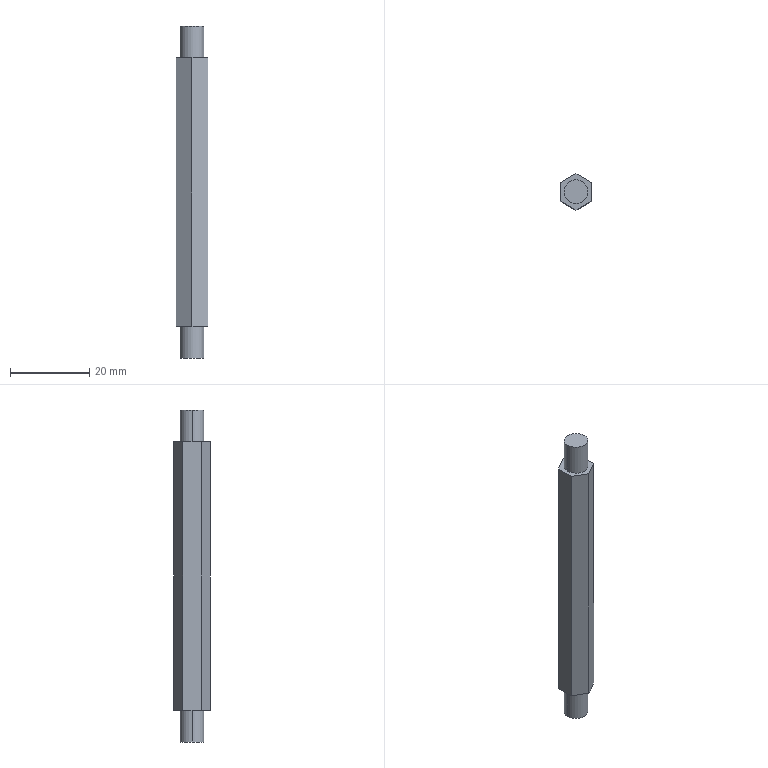Part | STEP file | 1 solid | 14 faces | box 8 x 9.238 x 84 mm | volume 4221 mm3 | plane 10 | cylinder 4 | commonest cylinder face diameters 6 x4
STEP:
#1=CARTESIAN_POINT('',(0.,0.,0.));
#2=DIRECTION('',(0.,0.,1.));
#3=DIRECTION('',(1.,0.,0.));
#4=AXIS2_PLACEMENT_3D('',#1,#2,#3);
#5=CARTESIAN_POINT('',(-5.42,-20.574,-52.535));
#6=VERTEX_POINT('',#5);
#7=CARTESIAN_POINT('',(-11.42,-20.574,-52.535));
#8=VERTEX_POINT('',#7);
#9=CARTESIAN_POINT('',(-8.42,-20.574,-52.535));
#10=DIRECTION('',(0.,0.,1.));
#11=DIRECTION('',(-1.,0.,0.));
#12=AXIS2_PLACEMENT_3D('',#9,#10,#11);
#13=CIRCLE('',#12,3.);
#14=CARTESIAN_POINT('',(-8.42,-20.574,-52.535));
#15=DIRECTION('',(0.,0.,-1.));
#16=DIRECTION('',(-1.,0.,0.));
#17=AXIS2_PLACEMENT_3D('',#14,#15,#16);
#18=CYLINDRICAL_SURFACE('',#17,3.);
#19=CARTESIAN_POINT('',(6.283,0.));
#20=DIRECTION('',(-1.,0.));
#21=VECTOR('',#20,1.);
#22=LINE('',#19,#21);
#23=(GEOMETRIC_REPRESENTATION_CONTEXT(2)PARAMETRIC_REPRESENTATION_CONTEXT()REPRESENTATION_CONTEXT('',''));
#24=DEFINITIONAL_REPRESENTATION('',(#22),#23);
#25=PCURVE('',#18,#24);
#26=CARTESIAN_POINT('',(-8.42,-20.574,-52.535));
#27=DIRECTION('',(0.,0.,-1.));
#28=DIRECTION('',(-1.,0.,0.));
#29=AXIS2_PLACEMENT_3D('',#26,#27,#28);
#30=PLANE('',#29);
#31=CARTESIAN_POINT('',(3.,0.));
#32=CARTESIAN_POINT('',(3.,-5.196));
#33=CARTESIAN_POINT('',(-1.5,-2.598));
#34=CARTESIAN_POINT('',(-6.,0.));
#35=CARTESIAN_POINT('',(-1.5,2.598));
#36=CARTESIAN_POINT('',(3.,5.196));
#37=CARTESIAN_POINT('',(3.,0.));
#38=(BOUNDED_CURVE()B_SPLINE_CURVE(2,(#31,#32,#33,#34,#35,#36,#37),.UNSPECIFIED.,.T.,.F.)B_SPLINE_CURVE_WITH_KNOTS((1,2,2,2,2,1),(-2.094,0.,2.094,4.189,6.283,8.378),.UNSPECIFIED.)CURVE()GEOMETRIC_REPRESENTATION_ITEM()RATIONAL_B_SPLINE_CURVE((1.,0.5,1.,0.5,1.,0.5,1.))REPRESENTATION_ITEM(''));
#39=(GEOMETRIC_REPRESENTATION_CONTEXT(2)PARAMETRIC_REPRESENTATION_CONTEXT()REPRESENTATION_CONTEXT('',''));
#40=DEFINITIONAL_REPRESENTATION('',(#38),#39);
#41=PCURVE('',#30,#40);
#42=SURFACE_CURVE('',#13,(#25,#41),.PCURVE_S1.);
#43=EDGE_CURVE('',#6,#8,#42,.T.);
#44=ORIENTED_EDGE('',*,*,#43,.F.);
#45=CARTESIAN_POINT('',(-5.42,-20.574,-60.535));
#46=VERTEX_POINT('',#45);
#47=CARTESIAN_POINT('',(-5.42,-20.574,-52.535));
#48=DIRECTION('',(0.,0.,-1.));
#49=VECTOR('',#48,1.);
#50=LINE('',#47,#49);
#51=CARTESIAN_POINT('',(3.142,0.));
#52=DIRECTION('',(0.,1.));
#53=VECTOR('',#52,1.);
#54=LINE('',#51,#53);
#55=(GEOMETRIC_REPRESENTATION_CONTEXT(2)PARAMETRIC_REPRESENTATION_CONTEXT()REPRESENTATION_CONTEXT('',''));
#56=DEFINITIONAL_REPRESENTATION('',(#54),#55);
#57=PCURVE('',#18,#56);
#58=CARTESIAN_POINT('',(-8.42,-20.574,-52.535));
#59=DIRECTION('',(0.,0.,-1.));
#60=DIRECTION('',(-1.,0.,0.));
#61=AXIS2_PLACEMENT_3D('',#58,#59,#60);
#62=CYLINDRICAL_SURFACE('',#61,3.);
#63=CARTESIAN_POINT('',(3.142,0.));
#64=DIRECTION('',(0.,1.));
#65=VECTOR('',#64,1.);
#66=LINE('',#63,#65);
#67=(GEOMETRIC_REPRESENTATION_CONTEXT(2)PARAMETRIC_REPRESENTATION_CONTEXT()REPRESENTATION_CONTEXT('',''));
#68=DEFINITIONAL_REPRESENTATION('',(#66),#67);
#69=PCURVE('',#62,#68);
#70=SURFACE_CURVE('',#50,(#57,#69),.PCURVE_S1.);
#71=EDGE_CURVE('',#6,#46,#70,.T.);
#72=ORIENTED_EDGE('',*,*,#71,.T.);
#73=CARTESIAN_POINT('',(-11.42,-20.574,-60.535));
#74=VERTEX_POINT('',#73);
#75=CARTESIAN_POINT('',(-8.42,-20.574,-60.535));
#76=DIRECTION('',(0.,0.,1.));
#77=DIRECTION('',(-1.,0.,0.));
#78=AXIS2_PLACEMENT_3D('',#75,#76,#77);
#79=CIRCLE('',#78,3.);
#80=CARTESIAN_POINT('',(6.283,8.));
#81=DIRECTION('',(-1.,0.));
#82=VECTOR('',#81,1.);
#83=LINE('',#80,#82);
#84=(GEOMETRIC_REPRESENTATION_CONTEXT(2)PARAMETRIC_REPRESENTATION_CONTEXT()REPRESENTATION_CONTEXT('',''));
#85=DEFINITIONAL_REPRESENTATION('',(#83),#84);
#86=PCURVE('',#18,#85);
#87=CARTESIAN_POINT('',(-8.42,-20.574,-60.535));
#88=DIRECTION('',(0.,0.,-1.));
#89=DIRECTION('',(0.,1.,0.));
#90=AXIS2_PLACEMENT_3D('',#87,#88,#89);
#91=PLANE('',#90);
#92=CARTESIAN_POINT('',(0.,-3.));
#93=CARTESIAN_POINT('',(-5.196,-3.));
#94=CARTESIAN_POINT('',(-2.598,1.5));
#95=CARTESIAN_POINT('',(0.,6.));
#96=CARTESIAN_POINT('',(2.598,1.5));
#97=CARTESIAN_POINT('',(5.196,-3.));
#98=CARTESIAN_POINT('',(0.,-3.));
#99=(BOUNDED_CURVE()B_SPLINE_CURVE(2,(#92,#93,#94,#95,#96,#97,#98),.UNSPECIFIED.,.T.,.F.)B_SPLINE_CURVE_WITH_KNOTS((1,2,2,2,2,1),(-2.094,0.,2.094,4.189,6.283,8.378),.UNSPECIFIED.)CURVE()GEOMETRIC_REPRESENTATION_ITEM()RATIONAL_B_SPLINE_CURVE((1.,0.5,1.,0.5,1.,0.5,1.))REPRESENTATION_ITEM(''));
#100=(GEOMETRIC_REPRESENTATION_CONTEXT(2)PARAMETRIC_REPRESENTATION_CONTEXT()REPRESENTATION_CONTEXT('',''));
#101=DEFINITIONAL_REPRESENTATION('',(#99),#100);
#102=PCURVE('',#91,#101);
#103=SURFACE_CURVE('',#79,(#86,#102),.PCURVE_S1.);
#104=EDGE_CURVE('',#46,#74,#103,.T.);
#105=ORIENTED_EDGE('',*,*,#104,.T.);
#106=CARTESIAN_POINT('',(-11.42,-20.574,-52.535));
#107=DIRECTION('',(0.,0.,-1.));
#108=VECTOR('',#107,1.);
#109=LINE('',#106,#108);
#110=CARTESIAN_POINT('',(0.,0.));
#111=DIRECTION('',(0.,1.));
#112=VECTOR('',#111,1.);
#113=LINE('',#110,#112);
#114=(GEOMETRIC_REPRESENTATION_CONTEXT(2)PARAMETRIC_REPRESENTATION_CONTEXT()REPRESENTATION_CONTEXT('',''));
#115=DEFINITIONAL_REPRESENTATION('',(#113),#114);
#116=PCURVE('',#18,#115);
#117=CARTESIAN_POINT('',(6.283,0.));
#118=DIRECTION('',(0.,1.));
#119=VECTOR('',#118,1.);
#120=LINE('',#117,#119);
#121=(GEOMETRIC_REPRESENTATION_CONTEXT(2)PARAMETRIC_REPRESENTATION_CONTEXT()REPRESENTATION_CONTEXT('',''));
#122=DEFINITIONAL_REPRESENTATION('',(#120),#121);
#123=PCURVE('',#62,#122);
#124=SURFACE_CURVE('',#109,(#116,#123),.PCURVE_S1.);
#125=EDGE_CURVE('',#8,#74,#124,.T.);
#126=ORIENTED_EDGE('',*,*,#125,.F.);
#127=EDGE_LOOP('',(#44,#72,#105,#126));
#128=FACE_BOUND('',#127,.T.);
#129=ADVANCED_FACE('',(#128),#18,.T.);
#130=CARTESIAN_POINT('',(-11.42,-20.574,23.465));
#131=VERTEX_POINT('',#130);
#132=CARTESIAN_POINT('',(-5.42,-20.574,23.465));
#133=VERTEX_POINT('',#132);
#134=CARTESIAN_POINT('',(-8.42,-20.574,23.465));
#135=DIRECTION('',(0.,0.,-1.));
#136=DIRECTION('',(-1.,0.,0.));
#137=AXIS2_PLACEMENT_3D('',#134,#135,#136);
#138=CIRCLE('',#137,3.);
#139=CARTESIAN_POINT('',(-8.42,-20.574,15.465));
#140=DIRECTION('',(0.,0.,-1.));
#141=DIRECTION('',(-1.,0.,0.));
#142=AXIS2_PLACEMENT_3D('',#139,#140,#141);
#143=CYLINDRICAL_SURFACE('',#142,3.);
#144=CARTESIAN_POINT('',(0.,-8.));
#145=DIRECTION('',(1.,0.));
#146=VECTOR('',#145,1.);
#147=LINE('',#144,#146);
#148=(GEOMETRIC_REPRESENTATION_CONTEXT(2)PARAMETRIC_REPRESENTATION_CONTEXT()REPRESENTATION_CONTEXT('',''));
#149=DEFINITIONAL_REPRESENTATION('',(#147),#148);
#150=PCURVE('',#143,#149);
#151=CARTESIAN_POINT('',(-8.42,-20.574,23.465));
#152=DIRECTION('',(0.,0.,-1.));
#153=DIRECTION('',(0.,1.,0.));
#154=AXIS2_PLACEMENT_3D('',#151,#152,#153);
#155=PLANE('',#154);
#156=CARTESIAN_POINT('',(0.,0.));
#157=DIRECTION('',(0.,-1.));
#158=AXIS2_PLACEMENT_2D('',#156,#157);
#159=CIRCLE('',#158,3.);
#160=(GEOMETRIC_REPRESENTATION_CONTEXT(2)PARAMETRIC_REPRESENTATION_CONTEXT()REPRESENTATION_CONTEXT('',''));
#161=DEFINITIONAL_REPRESENTATION('',(#159),#160);
#162=PCURVE('',#155,#161);
#163=SURFACE_CURVE('',#138,(#150,#162),.PCURVE_S1.);
#164=EDGE_CURVE('',#131,#133,#163,.T.);
#165=ORIENTED_EDGE('',*,*,#164,.T.);
#166=CARTESIAN_POINT('',(-5.42,-20.574,15.465));
#167=VERTEX_POINT('',#166);
#168=CARTESIAN_POINT('',(-5.42,-20.574,15.465));
#169=DIRECTION('',(0.,0.,-1.));
#170=VECTOR('',#169,1.);
#171=LINE('',#168,#170);
#172=CARTESIAN_POINT('',(3.142,0.));
#173=DIRECTION('',(0.,1.));
#174=VECTOR('',#173,1.);
#175=LINE('',#172,#174);
#176=(GEOMETRIC_REPRESENTATION_CONTEXT(2)PARAMETRIC_REPRESENTATION_CONTEXT()REPRESENTATION_CONTEXT('',''));
#177=DEFINITIONAL_REPRESENTATION('',(#175),#176);
#178=PCURVE('',#143,#177);
#179=CARTESIAN_POINT('',(-8.42,-20.574,15.465));
#180=DIRECTION('',(0.,0.,-1.));
#181=DIRECTION('',(-1.,0.,0.));
#182=AXIS2_PLACEMENT_3D('',#179,#180,#181);
#183=CYLINDRICAL_SURFACE('',#182,3.);
#184=CARTESIAN_POINT('',(3.142,0.));
#185=DIRECTION('',(0.,1.));
#186=VECTOR('',#185,1.);
#187=LINE('',#184,#186);
#188=(GEOMETRIC_REPRESENTATION_CONTEXT(2)PARAMETRIC_REPRESENTATION_CONTEXT()REPRESENTATION_CONTEXT('',''));
#189=DEFINITIONAL_REPRESENTATION('',(#187),#188);
#190=PCURVE('',#183,#189);
#191=SURFACE_CURVE('',#171,(#178,#190),.PCURVE_S1.);
#192=EDGE_CURVE('',#133,#167,#191,.T.);
#193=ORIENTED_EDGE('',*,*,#192,.T.);
#194=CARTESIAN_POINT('',(-11.42,-20.574,15.465));
#195=VERTEX_POINT('',#194);
#196=CARTESIAN_POINT('',(-8.42,-20.574,15.465));
#197=DIRECTION('',(0.,0.,-1.));
#198=DIRECTION('',(-1.,0.,0.));
#199=AXIS2_PLACEMENT_3D('',#196,#197,#198);
#200=CIRCLE('',#199,3.);
#201=CARTESIAN_POINT('',(0.,0.));
#202=DIRECTION('',(1.,0.));
#203=VECTOR('',#202,1.);
#204=LINE('',#201,#203);
#205=(GEOMETRIC_REPRESENTATION_CONTEXT(2)PARAMETRIC_REPRESENTATION_CONTEXT()REPRESENTATION_CONTEXT('',''));
#206=DEFINITIONAL_REPRESENTATION('',(#204),#205);
#207=PCURVE('',#143,#206);
#208=CARTESIAN_POINT('',(-8.42,-20.574,15.465));
#209=DIRECTION('',(0.,0.,1.));
#210=DIRECTION('',(1.,0.,0.));
#211=AXIS2_PLACEMENT_3D('',#208,#209,#210);
#212=PLANE('',#211);
#213=CARTESIAN_POINT('',(-3.,0.));
#214=CARTESIAN_POINT('',(-3.,5.196));
#215=CARTESIAN_POINT('',(1.5,2.598));
#216=CARTESIAN_POINT('',(6.,0.));
#217=CARTESIAN_POINT('',(1.5,-2.598));
#218=CARTESIAN_POINT('',(-3.,-5.196));
#219=CARTESIAN_POINT('',(-3.,0.));
#220=(BOUNDED_CURVE()B_SPLINE_CURVE(2,(#213,#214,#215,#216,#217,#218,#219),.UNSPECIFIED.,.T.,.F.)B_SPLINE_CURVE_WITH_KNOTS((1,2,2,2,2,1),(-2.094,0.,2.094,4.189,6.283,8.378),.UNSPECIFIED.)CURVE()GEOMETRIC_REPRESENTATION_ITEM()RATIONAL_B_SPLINE_CURVE((1.,0.5,1.,0.5,1.,0.5,1.))REPRESENTATION_ITEM(''));
#221=(GEOMETRIC_REPRESENTATION_CONTEXT(2)PARAMETRIC_REPRESENTATION_CONTEXT()REPRESENTATION_CONTEXT('',''));
#222=DEFINITIONAL_REPRESENTATION('',(#220),#221);
#223=PCURVE('',#212,#222);
#224=SURFACE_CURVE('',#200,(#207,#223),.PCURVE_S1.);
#225=EDGE_CURVE('',#195,#167,#224,.T.);
#226=ORIENTED_EDGE('',*,*,#225,.F.);
#227=CARTESIAN_POINT('',(-11.42,-20.574,15.465));
#228=DIRECTION('',(0.,0.,-1.));
#229=VECTOR('',#228,1.);
#230=LINE('',#227,#229);
#231=CARTESIAN_POINT('',(0.,0.));
#232=DIRECTION('',(0.,1.));
#233=VECTOR('',#232,1.);
#234=LINE('',#231,#233);
#235=(GEOMETRIC_REPRESENTATION_CONTEXT(2)PARAMETRIC_REPRESENTATION_CONTEXT()REPRESENTATION_CONTEXT('',''));
#236=DEFINITIONAL_REPRESENTATION('',(#234),#235);
#237=PCURVE('',#143,#236);
#238=CARTESIAN_POINT('',(6.283,0.));
#239=DIRECTION('',(0.,1.));
#240=VECTOR('',#239,1.);
#241=LINE('',#238,#240);
#242=(GEOMETRIC_REPRESENTATION_CONTEXT(2)PARAMETRIC_REPRESENTATION_CONTEXT()REPRESENTATION_CONTEXT('',''));
#243=DEFINITIONAL_REPRESENTATION('',(#241),#242);
#244=PCURVE('',#183,#243);
#245=SURFACE_CURVE('',#230,(#237,#244),.PCURVE_S1.);
#246=EDGE_CURVE('',#131,#195,#245,.T.);
#247=ORIENTED_EDGE('',*,*,#246,.F.);
#248=EDGE_LOOP('',(#165,#193,#226,#247));
#249=FACE_BOUND('',#248,.T.);
#250=ADVANCED_FACE('',(#249),#143,.T.);
#251=CARTESIAN_POINT('',(-8.42,-25.193,15.465));
#252=VERTEX_POINT('',#251);
#253=CARTESIAN_POINT('',(-8.42,-25.193,-52.535));
#254=VERTEX_POINT('',#253);
#255=CARTESIAN_POINT('',(-8.42,-25.193,-18.535));
#256=DIRECTION('',(0.,0.,-1.));
#257=VECTOR('',#256,1.);
#258=LINE('',#255,#257);
#259=CARTESIAN_POINT('',(-8.42,-25.193,-18.535));
#260=DIRECTION('',(0.5,-0.866,0.));
#261=DIRECTION('',(0.866,0.5,0.));
#262=AXIS2_PLACEMENT_3D('',#259,#260,#261);
#263=PLANE('',#262);
#264=CARTESIAN_POINT('',(0.,0.));
#265=DIRECTION('',(0.,-1.));
#266=VECTOR('',#265,1.);
#267=LINE('',#264,#266);
#268=(GEOMETRIC_REPRESENTATION_CONTEXT(2)PARAMETRIC_REPRESENTATION_CONTEXT()REPRESENTATION_CONTEXT('',''));
#269=DEFINITIONAL_REPRESENTATION('',(#267),#268);
#270=PCURVE('',#263,#269);
#271=CARTESIAN_POINT('',(-12.42,-22.883,-18.535));
#272=DIRECTION('',(-0.5,-0.866,0.));
#273=DIRECTION('',(0.866,-0.5,0.));
#274=AXIS2_PLACEMENT_3D('',#271,#272,#273);
#275=PLANE('',#274);
#276=CARTESIAN_POINT('',(4.619,0.));
#277=DIRECTION('',(0.,-1.));
#278=VECTOR('',#277,1.);
#279=LINE('',#276,#278);
#280=(GEOMETRIC_REPRESENTATION_CONTEXT(2)PARAMETRIC_REPRESENTATION_CONTEXT()REPRESENTATION_CONTEXT('',''));
#281=DEFINITIONAL_REPRESENTATION('',(#279),#280);
#282=PCURVE('',#275,#281);
#283=SURFACE_CURVE('',#258,(#270,#282),.PCURVE_S1.);
#284=EDGE_CURVE('',#252,#254,#283,.T.);
#285=ORIENTED_EDGE('',*,*,#284,.T.);
#286=CARTESIAN_POINT('',(-4.42,-22.883,-52.535));
#287=VERTEX_POINT('',#286);
#288=CARTESIAN_POINT('',(-8.42,-25.193,-52.535));
#289=DIRECTION('',(0.866,0.5,0.));
#290=VECTOR('',#289,1.);
#291=LINE('',#288,#290);
#292=CARTESIAN_POINT('',(0.,-34.));
#293=DIRECTION('',(1.,0.));
#294=VECTOR('',#293,1.);
#295=LINE('',#292,#294);
#296=(GEOMETRIC_REPRESENTATION_CONTEXT(2)PARAMETRIC_REPRESENTATION_CONTEXT()REPRESENTATION_CONTEXT('',''));
#297=DEFINITIONAL_REPRESENTATION('',(#295),#296);
#298=PCURVE('',#263,#297);
#299=CARTESIAN_POINT('',(0.,-4.619));
#300=DIRECTION('',(-0.866,0.5));
#301=VECTOR('',#300,1.);
#302=LINE('',#299,#301);
#303=(GEOMETRIC_REPRESENTATION_CONTEXT(2)PARAMETRIC_REPRESENTATION_CONTEXT()REPRESENTATION_CONTEXT('',''));
#304=DEFINITIONAL_REPRESENTATION('',(#302),#303);
#305=PCURVE('',#30,#304);
#306=SURFACE_CURVE('',#291,(#298,#305),.PCURVE_S1.);
#307=EDGE_CURVE('',#254,#287,#306,.T.);
#308=ORIENTED_EDGE('',*,*,#307,.T.);
#309=CARTESIAN_POINT('',(-4.42,-22.883,15.465));
#310=VERTEX_POINT('',#309);
#311=CARTESIAN_POINT('',(-4.42,-22.883,-18.535));
#312=DIRECTION('',(0.,0.,1.));
#313=VECTOR('',#312,1.);
#314=LINE('',#311,#313);
#315=CARTESIAN_POINT('',(4.619,0.));
#316=DIRECTION('',(0.,1.));
#317=VECTOR('',#316,1.);
#318=LINE('',#315,#317);
#319=(GEOMETRIC_REPRESENTATION_CONTEXT(2)PARAMETRIC_REPRESENTATION_CONTEXT()REPRESENTATION_CONTEXT('',''));
#320=DEFINITIONAL_REPRESENTATION('',(#318),#319);
#321=PCURVE('',#263,#320);
#322=CARTESIAN_POINT('',(-4.42,-22.883,-18.535));
#323=DIRECTION('',(1.,0.,0.));
#324=DIRECTION('',(0.,1.,0.));
#325=AXIS2_PLACEMENT_3D('',#322,#323,#324);
#326=PLANE('',#325);
#327=CARTESIAN_POINT('',(0.,0.));
#328=DIRECTION('',(0.,1.));
#329=VECTOR('',#328,1.);
#330=LINE('',#327,#329);
#331=(GEOMETRIC_REPRESENTATION_CONTEXT(2)PARAMETRIC_REPRESENTATION_CONTEXT()REPRESENTATION_CONTEXT('',''));
#332=DEFINITIONAL_REPRESENTATION('',(#330),#331);
#333=PCURVE('',#326,#332);
#334=SURFACE_CURVE('',#314,(#321,#333),.PCURVE_S1.);
#335=EDGE_CURVE('',#287,#310,#334,.T.);
#336=ORIENTED_EDGE('',*,*,#335,.T.);
#337=CARTESIAN_POINT('',(-8.42,-25.193,15.465));
#338=DIRECTION('',(-0.866,-0.5,0.));
#339=VECTOR('',#338,1.);
#340=LINE('',#337,#339);
#341=CARTESIAN_POINT('',(0.,34.));
#342=DIRECTION('',(-1.,0.));
#343=VECTOR('',#342,1.);
#344=LINE('',#341,#343);
#345=(GEOMETRIC_REPRESENTATION_CONTEXT(2)PARAMETRIC_REPRESENTATION_CONTEXT()REPRESENTATION_CONTEXT('',''));
#346=DEFINITIONAL_REPRESENTATION('',(#344),#345);
#347=PCURVE('',#263,#346);
#348=CARTESIAN_POINT('',(0.,-4.619));
#349=DIRECTION('',(-0.866,-0.5));
#350=VECTOR('',#349,1.);
#351=LINE('',#348,#350);
#352=(GEOMETRIC_REPRESENTATION_CONTEXT(2)PARAMETRIC_REPRESENTATION_CONTEXT()REPRESENTATION_CONTEXT('',''));
#353=DEFINITIONAL_REPRESENTATION('',(#351),#352);
#354=PCURVE('',#212,#353);
#355=SURFACE_CURVE('',#340,(#347,#354),.PCURVE_S1.);
#356=EDGE_CURVE('',#310,#252,#355,.T.);
#357=ORIENTED_EDGE('',*,*,#356,.T.);
#358=EDGE_LOOP('',(#285,#308,#336,#357));
#359=FACE_BOUND('',#358,.T.);
#360=ADVANCED_FACE('',(#359),#263,.T.);
#361=CARTESIAN_POINT('',(-12.42,-22.883,-52.535));
#362=VERTEX_POINT('',#361);
#363=CARTESIAN_POINT('',(-8.42,-25.193,-52.535));
#364=DIRECTION('',(-0.866,0.5,0.));
#365=VECTOR('',#364,1.);
#366=LINE('',#363,#365);
#367=CARTESIAN_POINT('',(0.,-4.619));
#368=DIRECTION('',(0.866,0.5));
#369=VECTOR('',#368,1.);
#370=LINE('',#367,#369);
#371=(GEOMETRIC_REPRESENTATION_CONTEXT(2)PARAMETRIC_REPRESENTATION_CONTEXT()REPRESENTATION_CONTEXT('',''));
#372=DEFINITIONAL_REPRESENTATION('',(#370),#371);
#373=PCURVE('',#30,#372);
#374=CARTESIAN_POINT('',(4.619,-34.));
#375=DIRECTION('',(-1.,0.));
#376=VECTOR('',#375,1.);
#377=LINE('',#374,#376);
#378=(GEOMETRIC_REPRESENTATION_CONTEXT(2)PARAMETRIC_REPRESENTATION_CONTEXT()REPRESENTATION_CONTEXT('',''));
#379=DEFINITIONAL_REPRESENTATION('',(#377),#378);
#380=PCURVE('',#275,#379);
#381=SURFACE_CURVE('',#366,(#373,#380),.PCURVE_S1.);
#382=EDGE_CURVE('',#254,#362,#381,.T.);
#383=ORIENTED_EDGE('',*,*,#382,.T.);
#384=CARTESIAN_POINT('',(-12.42,-18.264,-52.535));
#385=VERTEX_POINT('',#384);
#386=CARTESIAN_POINT('',(-12.42,-20.574,-52.535));
#387=DIRECTION('',(0.,1.,0.));
#388=VECTOR('',#387,1.);
#389=LINE('',#386,#388);
#390=CARTESIAN_POINT('',(4.,0.));
#391=DIRECTION('',(0.,1.));
#392=VECTOR('',#391,1.);
#393=LINE('',#390,#392);
#394=(GEOMETRIC_REPRESENTATION_CONTEXT(2)PARAMETRIC_REPRESENTATION_CONTEXT()REPRESENTATION_CONTEXT('',''));
#395=DEFINITIONAL_REPRESENTATION('',(#393),#394);
#396=PCURVE('',#30,#395);
#397=CARTESIAN_POINT('',(-12.42,-18.264,-18.535));
#398=DIRECTION('',(-1.,0.,0.));
#399=DIRECTION('',(0.,-1.,0.));
#400=AXIS2_PLACEMENT_3D('',#397,#398,#399);
#401=PLANE('',#400);
#402=CARTESIAN_POINT('',(2.309,-34.));
#403=DIRECTION('',(-1.,0.));
#404=VECTOR('',#403,1.);
#405=LINE('',#402,#404);
#406=(GEOMETRIC_REPRESENTATION_CONTEXT(2)PARAMETRIC_REPRESENTATION_CONTEXT()REPRESENTATION_CONTEXT('',''));
#407=DEFINITIONAL_REPRESENTATION('',(#405),#406);
#408=PCURVE('',#401,#407);
#409=SURFACE_CURVE('',#389,(#396,#408),.PCURVE_S1.);
#410=EDGE_CURVE('',#362,#385,#409,.T.);
#411=ORIENTED_EDGE('',*,*,#410,.T.);
#412=CARTESIAN_POINT('',(-8.42,-15.955,-52.535));
#413=VERTEX_POINT('',#412);
#414=CARTESIAN_POINT('',(-12.42,-18.264,-52.535));
#415=DIRECTION('',(0.866,0.5,0.));
#416=VECTOR('',#415,1.);
#417=LINE('',#414,#416);
#418=CARTESIAN_POINT('',(4.,2.309));
#419=DIRECTION('',(-0.866,0.5));
#420=VECTOR('',#419,1.);
#421=LINE('',#418,#420);
#422=(GEOMETRIC_REPRESENTATION_CONTEXT(2)PARAMETRIC_REPRESENTATION_CONTEXT()REPRESENTATION_CONTEXT('',''));
#423=DEFINITIONAL_REPRESENTATION('',(#421),#422);
#424=PCURVE('',#30,#423);
#425=CARTESIAN_POINT('',(-8.42,-15.955,-18.535));
#426=DIRECTION('',(-0.5,0.866,0.));
#427=DIRECTION('',(-0.866,-0.5,0.));
#428=AXIS2_PLACEMENT_3D('',#425,#426,#427);
#429=PLANE('',#428);
#430=CARTESIAN_POINT('',(4.619,-34.));
#431=DIRECTION('',(-1.,0.));
#432=VECTOR('',#431,1.);
#433=LINE('',#430,#432);
#434=(GEOMETRIC_REPRESENTATION_CONTEXT(2)PARAMETRIC_REPRESENTATION_CONTEXT()REPRESENTATION_CONTEXT('',''));
#435=DEFINITIONAL_REPRESENTATION('',(#433),#434);
#436=PCURVE('',#429,#435);
#437=SURFACE_CURVE('',#417,(#424,#436),.PCURVE_S1.);
#438=EDGE_CURVE('',#385,#413,#437,.T.);
#439=ORIENTED_EDGE('',*,*,#438,.T.);
#440=CARTESIAN_POINT('',(-4.42,-18.264,-52.535));
#441=VERTEX_POINT('',#440);
#442=CARTESIAN_POINT('',(-8.42,-15.955,-52.535));
#443=DIRECTION('',(0.866,-0.5,0.));
#444=VECTOR('',#443,1.);
#445=LINE('',#442,#444);
#446=CARTESIAN_POINT('',(0.,4.619));
#447=DIRECTION('',(-0.866,-0.5));
#448=VECTOR('',#447,1.);
#449=LINE('',#446,#448);
#450=(GEOMETRIC_REPRESENTATION_CONTEXT(2)PARAMETRIC_REPRESENTATION_CONTEXT()REPRESENTATION_CONTEXT('',''));
#451=DEFINITIONAL_REPRESENTATION('',(#449),#450);
#452=PCURVE('',#30,#451);
#453=CARTESIAN_POINT('',(-4.42,-18.264,-18.535));
#454=DIRECTION('',(0.5,0.866,0.));
#455=DIRECTION('',(-0.866,0.5,0.));
#456=AXIS2_PLACEMENT_3D('',#453,#454,#455);
#457=PLANE('',#456);
#458=CARTESIAN_POINT('',(4.619,-34.));
#459=DIRECTION('',(-1.,0.));
#460=VECTOR('',#459,1.);
#461=LINE('',#458,#460);
#462=(GEOMETRIC_REPRESENTATION_CONTEXT(2)PARAMETRIC_REPRESENTATION_CONTEXT()REPRESENTATION_CONTEXT('',''));
#463=DEFINITIONAL_REPRESENTATION('',(#461),#462);
#464=PCURVE('',#457,#463);
#465=SURFACE_CURVE('',#445,(#452,#464),.PCURVE_S1.);
#466=EDGE_CURVE('',#413,#441,#465,.T.);
#467=ORIENTED_EDGE('',*,*,#466,.T.);
#468=CARTESIAN_POINT('',(-4.42,-20.574,-52.535));
#469=DIRECTION('',(0.,-1.,0.));
#470=VECTOR('',#469,1.);
#471=LINE('',#468,#470);
#472=CARTESIAN_POINT('',(-4.,0.));
#473=DIRECTION('',(0.,-1.));
#474=VECTOR('',#473,1.);
#475=LINE('',#472,#474);
#476=(GEOMETRIC_REPRESENTATION_CONTEXT(2)PARAMETRIC_REPRESENTATION_CONTEXT()REPRESENTATION_CONTEXT('',''));
#477=DEFINITIONAL_REPRESENTATION('',(#475),#476);
#478=PCURVE('',#30,#477);
#479=CARTESIAN_POINT('',(2.309,-34.));
#480=DIRECTION('',(-1.,0.));
#481=VECTOR('',#480,1.);
#482=LINE('',#479,#481);
#483=(GEOMETRIC_REPRESENTATION_CONTEXT(2)PARAMETRIC_REPRESENTATION_CONTEXT()REPRESENTATION_CONTEXT('',''));
#484=DEFINITIONAL_REPRESENTATION('',(#482),#483);
#485=PCURVE('',#326,#484);
#486=SURFACE_CURVE('',#471,(#478,#485),.PCURVE_S1.);
#487=EDGE_CURVE('',#441,#287,#486,.T.);
#488=ORIENTED_EDGE('',*,*,#487,.T.);
#489=ORIENTED_EDGE('',*,*,#307,.F.);
#490=EDGE_LOOP('',(#383,#411,#439,#467,#488,#489));
#491=FACE_BOUND('',#490,.T.);
#492=CARTESIAN_POINT('',(-8.42,-20.574,-52.535));
#493=DIRECTION('',(0.,0.,1.));
#494=DIRECTION('',(-1.,0.,0.));
#495=AXIS2_PLACEMENT_3D('',#492,#493,#494);
#496=CIRCLE('',#495,3.);
#497=CARTESIAN_POINT('',(3.,0.));
#498=CARTESIAN_POINT('',(3.,-5.196));
#499=CARTESIAN_POINT('',(-1.5,-2.598));
#500=CARTESIAN_POINT('',(-6.,0.));
#501=CARTESIAN_POINT('',(-1.5,2.598));
#502=CARTESIAN_POINT('',(3.,5.196));
#503=CARTESIAN_POINT('',(3.,0.));
#504=(BOUNDED_CURVE()B_SPLINE_CURVE(2,(#497,#498,#499,#500,#501,#502,#503),.UNSPECIFIED.,.T.,.F.)B_SPLINE_CURVE_WITH_KNOTS((1,2,2,2,2,1),(-2.094,0.,2.094,4.189,6.283,8.378),.UNSPECIFIED.)CURVE()GEOMETRIC_REPRESENTATION_ITEM()RATIONAL_B_SPLINE_CURVE((1.,0.5,1.,0.5,1.,0.5,1.))REPRESENTATION_ITEM(''));
#505=(GEOMETRIC_REPRESENTATION_CONTEXT(2)PARAMETRIC_REPRESENTATION_CONTEXT()REPRESENTATION_CONTEXT('',''));
#506=DEFINITIONAL_REPRESENTATION('',(#504),#505);
#507=PCURVE('',#30,#506);
#508=CARTESIAN_POINT('',(6.283,0.));
#509=DIRECTION('',(-1.,0.));
#510=VECTOR('',#509,1.);
#511=LINE('',#508,#510);
#512=(GEOMETRIC_REPRESENTATION_CONTEXT(2)PARAMETRIC_REPRESENTATION_CONTEXT()REPRESENTATION_CONTEXT('',''));
#513=DEFINITIONAL_REPRESENTATION('',(#511),#512);
#514=PCURVE('',#62,#513);
#515=SURFACE_CURVE('',#496,(#507,#514),.PCURVE_S1.);
#516=EDGE_CURVE('',#8,#6,#515,.T.);
#517=ORIENTED_EDGE('',*,*,#516,.T.);
#518=ORIENTED_EDGE('',*,*,#43,.T.);
#519=EDGE_LOOP('',(#517,#518));
#520=FACE_BOUND('',#519,.T.);
#521=ADVANCED_FACE('',(#491,#520),#30,.T.);
#522=CARTESIAN_POINT('',(-12.42,-22.883,15.465));
#523=VERTEX_POINT('',#522);
#524=CARTESIAN_POINT('',(-12.42,-22.883,-18.535));
#525=DIRECTION('',(0.,0.,-1.));
#526=VECTOR('',#525,1.);
#527=LINE('',#524,#526);
#528=CARTESIAN_POINT('',(0.,0.));
#529=DIRECTION('',(0.,-1.));
#530=VECTOR('',#529,1.);
#531=LINE('',#528,#530);
#532=(GEOMETRIC_REPRESENTATION_CONTEXT(2)PARAMETRIC_REPRESENTATION_CONTEXT()REPRESENTATION_CONTEXT('',''));
#533=DEFINITIONAL_REPRESENTATION('',(#531),#532);
#534=PCURVE('',#275,#533);
#535=CARTESIAN_POINT('',(4.619,0.));
#536=DIRECTION('',(0.,-1.));
#537=VECTOR('',#536,1.);
#538=LINE('',#535,#537);
#539=(GEOMETRIC_REPRESENTATION_CONTEXT(2)PARAMETRIC_REPRESENTATION_CONTEXT()REPRESENTATION_CONTEXT('',''));
#540=DEFINITIONAL_REPRESENTATION('',(#538),#539);
#541=PCURVE('',#401,#540);
#542=SURFACE_CURVE('',#527,(#534,#541),.PCURVE_S1.);
#543=EDGE_CURVE('',#523,#362,#542,.T.);
#544=ORIENTED_EDGE('',*,*,#543,.T.);
#545=ORIENTED_EDGE('',*,*,#382,.F.);
#546=ORIENTED_EDGE('',*,*,#284,.F.);
#547=CARTESIAN_POINT('',(-12.42,-22.883,15.465));
#548=DIRECTION('',(-0.866,0.5,0.));
#549=VECTOR('',#548,1.);
#550=LINE('',#547,#549);
#551=CARTESIAN_POINT('',(0.,34.));
#552=DIRECTION('',(-1.,0.));
#553=VECTOR('',#552,1.);
#554=LINE('',#551,#553);
#555=(GEOMETRIC_REPRESENTATION_CONTEXT(2)PARAMETRIC_REPRESENTATION_CONTEXT()REPRESENTATION_CONTEXT('',''));
#556=DEFINITIONAL_REPRESENTATION('',(#554),#555);
#557=PCURVE('',#275,#556);
#558=CARTESIAN_POINT('',(-4.,-2.309));
#559=DIRECTION('',(-0.866,0.5));
#560=VECTOR('',#559,1.);
#561=LINE('',#558,#560);
#562=(GEOMETRIC_REPRESENTATION_CONTEXT(2)PARAMETRIC_REPRESENTATION_CONTEXT()REPRESENTATION_CONTEXT('',''));
#563=DEFINITIONAL_REPRESENTATION('',(#561),#562);
#564=PCURVE('',#212,#563);
#565=SURFACE_CURVE('',#550,(#557,#564),.PCURVE_S1.);
#566=EDGE_CURVE('',#252,#523,#565,.T.);
#567=ORIENTED_EDGE('',*,*,#566,.T.);
#568=EDGE_LOOP('',(#544,#545,#546,#567));
#569=FACE_BOUND('',#568,.T.);
#570=ADVANCED_FACE('',(#569),#275,.T.);
#571=CARTESIAN_POINT('',(-4.42,-18.264,15.465));
#572=VERTEX_POINT('',#571);
#573=CARTESIAN_POINT('',(-4.42,-20.574,15.465));
#574=DIRECTION('',(0.,1.,0.));
#575=VECTOR('',#574,1.);
#576=LINE('',#573,#575);
#577=CARTESIAN_POINT('',(4.,0.));
#578=DIRECTION('',(0.,1.));
#579=VECTOR('',#578,1.);
#580=LINE('',#577,#579);
#581=(GEOMETRIC_REPRESENTATION_CONTEXT(2)PARAMETRIC_REPRESENTATION_CONTEXT()REPRESENTATION_CONTEXT('',''));
#582=DEFINITIONAL_REPRESENTATION('',(#580),#581);
#583=PCURVE('',#212,#582);
#584=CARTESIAN_POINT('',(2.309,34.));
#585=DIRECTION('',(1.,0.));
#586=VECTOR('',#585,1.);
#587=LINE('',#584,#586);
#588=(GEOMETRIC_REPRESENTATION_CONTEXT(2)PARAMETRIC_REPRESENTATION_CONTEXT()REPRESENTATION_CONTEXT('',''));
#589=DEFINITIONAL_REPRESENTATION('',(#587),#588);
#590=PCURVE('',#326,#589);
#591=SURFACE_CURVE('',#576,(#583,#590),.PCURVE_S1.);
#592=EDGE_CURVE('',#310,#572,#591,.T.);
#593=ORIENTED_EDGE('',*,*,#592,.T.);
#594=CARTESIAN_POINT('',(-8.42,-15.955,15.465));
#595=VERTEX_POINT('',#594);
#596=CARTESIAN_POINT('',(-4.42,-18.264,15.465));
#597=DIRECTION('',(-0.866,0.5,0.));
#598=VECTOR('',#597,1.);
#599=LINE('',#596,#598);
#600=CARTESIAN_POINT('',(4.,2.309));
#601=DIRECTION('',(-0.866,0.5));
#602=VECTOR('',#601,1.);
#603=LINE('',#600,#602);
#604=(GEOMETRIC_REPRESENTATION_CONTEXT(2)PARAMETRIC_REPRESENTATION_CONTEXT()REPRESENTATION_CONTEXT('',''));
#605=DEFINITIONAL_REPRESENTATION('',(#603),#604);
#606=PCURVE('',#212,#605);
#607=CARTESIAN_POINT('',(0.,34.));
#608=DIRECTION('',(1.,0.));
#609=VECTOR('',#608,1.);
#610=LINE('',#607,#609);
#611=(GEOMETRIC_REPRESENTATION_CONTEXT(2)PARAMETRIC_REPRESENTATION_CONTEXT()REPRESENTATION_CONTEXT('',''));
#612=DEFINITIONAL_REPRESENTATION('',(#610),#611);
#613=PCURVE('',#457,#612);
#614=SURFACE_CURVE('',#599,(#606,#613),.PCURVE_S1.);
#615=EDGE_CURVE('',#572,#595,#614,.T.);
#616=ORIENTED_EDGE('',*,*,#615,.T.);
#617=CARTESIAN_POINT('',(-12.42,-18.264,15.465));
#618=VERTEX_POINT('',#617);
#619=CARTESIAN_POINT('',(-8.42,-15.955,15.465));
#620=DIRECTION('',(-0.866,-0.5,0.));
#621=VECTOR('',#620,1.);
#622=LINE('',#619,#621);
#623=CARTESIAN_POINT('',(0.,4.619));
#624=DIRECTION('',(-0.866,-0.5));
#625=VECTOR('',#624,1.);
#626=LINE('',#623,#625);
#627=(GEOMETRIC_REPRESENTATION_CONTEXT(2)PARAMETRIC_REPRESENTATION_CONTEXT()REPRESENTATION_CONTEXT('',''));
#628=DEFINITIONAL_REPRESENTATION('',(#626),#627);
#629=PCURVE('',#212,#628);
#630=CARTESIAN_POINT('',(0.,34.));
#631=DIRECTION('',(1.,0.));
#632=VECTOR('',#631,1.);
#633=LINE('',#630,#632);
#634=(GEOMETRIC_REPRESENTATION_CONTEXT(2)PARAMETRIC_REPRESENTATION_CONTEXT()REPRESENTATION_CONTEXT('',''));
#635=DEFINITIONAL_REPRESENTATION('',(#633),#634);
#636=PCURVE('',#429,#635);
#637=SURFACE_CURVE('',#622,(#629,#636),.PCURVE_S1.);
#638=EDGE_CURVE('',#595,#618,#637,.T.);
#639=ORIENTED_EDGE('',*,*,#638,.T.);
#640=CARTESIAN_POINT('',(-12.42,-20.574,15.465));
#641=DIRECTION('',(0.,-1.,0.));
#642=VECTOR('',#641,1.);
#643=LINE('',#640,#642);
#644=CARTESIAN_POINT('',(-4.,0.));
#645=DIRECTION('',(0.,-1.));
#646=VECTOR('',#645,1.);
#647=LINE('',#644,#646);
#648=(GEOMETRIC_REPRESENTATION_CONTEXT(2)PARAMETRIC_REPRESENTATION_CONTEXT()REPRESENTATION_CONTEXT('',''));
#649=DEFINITIONAL_REPRESENTATION('',(#647),#648);
#650=PCURVE('',#212,#649);
#651=CARTESIAN_POINT('',(2.309,34.));
#652=DIRECTION('',(1.,0.));
#653=VECTOR('',#652,1.);
#654=LINE('',#651,#653);
#655=(GEOMETRIC_REPRESENTATION_CONTEXT(2)PARAMETRIC_REPRESENTATION_CONTEXT()REPRESENTATION_CONTEXT('',''));
#656=DEFINITIONAL_REPRESENTATION('',(#654),#655);
#657=PCURVE('',#401,#656);
#658=SURFACE_CURVE('',#643,(#650,#657),.PCURVE_S1.);
#659=EDGE_CURVE('',#618,#523,#658,.T.);
#660=ORIENTED_EDGE('',*,*,#659,.T.);
#661=ORIENTED_EDGE('',*,*,#566,.F.);
#662=ORIENTED_EDGE('',*,*,#356,.F.);
#663=EDGE_LOOP('',(#593,#616,#639,#660,#661,#662));
#664=FACE_BOUND('',#663,.T.);
#665=ORIENTED_EDGE('',*,*,#225,.T.);
#666=CARTESIAN_POINT('',(-8.42,-20.574,15.465));
#667=DIRECTION('',(0.,0.,-1.));
#668=DIRECTION('',(-1.,0.,0.));
#669=AXIS2_PLACEMENT_3D('',#666,#667,#668);
#670=CIRCLE('',#669,3.);
#671=CARTESIAN_POINT('',(-3.,0.));
#672=CARTESIAN_POINT('',(-3.,5.196));
#673=CARTESIAN_POINT('',(1.5,2.598));
#674=CARTESIAN_POINT('',(6.,0.));
#675=CARTESIAN_POINT('',(1.5,-2.598));
#676=CARTESIAN_POINT('',(-3.,-5.196));
#677=CARTESIAN_POINT('',(-3.,0.));
#678=(BOUNDED_CURVE()B_SPLINE_CURVE(2,(#671,#672,#673,#674,#675,#676,#677),.UNSPECIFIED.,.T.,.F.)B_SPLINE_CURVE_WITH_KNOTS((1,2,2,2,2,1),(-2.094,0.,2.094,4.189,6.283,8.378),.UNSPECIFIED.)CURVE()GEOMETRIC_REPRESENTATION_ITEM()RATIONAL_B_SPLINE_CURVE((1.,0.5,1.,0.5,1.,0.5,1.))REPRESENTATION_ITEM(''));
#679=(GEOMETRIC_REPRESENTATION_CONTEXT(2)PARAMETRIC_REPRESENTATION_CONTEXT()REPRESENTATION_CONTEXT('',''));
#680=DEFINITIONAL_REPRESENTATION('',(#678),#679);
#681=PCURVE('',#212,#680);
#682=CARTESIAN_POINT('',(0.,0.));
#683=DIRECTION('',(1.,0.));
#684=VECTOR('',#683,1.);
#685=LINE('',#682,#684);
#686=(GEOMETRIC_REPRESENTATION_CONTEXT(2)PARAMETRIC_REPRESENTATION_CONTEXT()REPRESENTATION_CONTEXT('',''));
#687=DEFINITIONAL_REPRESENTATION('',(#685),#686);
#688=PCURVE('',#183,#687);
#689=SURFACE_CURVE('',#670,(#681,#688),.PCURVE_S1.);
#690=EDGE_CURVE('',#167,#195,#689,.T.);
#691=ORIENTED_EDGE('',*,*,#690,.T.);
#692=EDGE_LOOP('',(#665,#691));
#693=FACE_BOUND('',#692,.T.);
#694=ADVANCED_FACE('',(#664,#693),#212,.T.);
#695=ORIENTED_EDGE('',*,*,#335,.F.);
#696=ORIENTED_EDGE('',*,*,#487,.F.);
#697=CARTESIAN_POINT('',(-4.42,-18.264,-18.535));
#698=DIRECTION('',(0.,0.,1.));
#699=VECTOR('',#698,1.);
#700=LINE('',#697,#699);
#701=CARTESIAN_POINT('',(4.619,0.));
#702=DIRECTION('',(0.,1.));
#703=VECTOR('',#702,1.);
#704=LINE('',#701,#703);
#705=(GEOMETRIC_REPRESENTATION_CONTEXT(2)PARAMETRIC_REPRESENTATION_CONTEXT()REPRESENTATION_CONTEXT('',''));
#706=DEFINITIONAL_REPRESENTATION('',(#704),#705);
#707=PCURVE('',#326,#706);
#708=CARTESIAN_POINT('',(0.,0.));
#709=DIRECTION('',(0.,1.));
#710=VECTOR('',#709,1.);
#711=LINE('',#708,#710);
#712=(GEOMETRIC_REPRESENTATION_CONTEXT(2)PARAMETRIC_REPRESENTATION_CONTEXT()REPRESENTATION_CONTEXT('',''));
#713=DEFINITIONAL_REPRESENTATION('',(#711),#712);
#714=PCURVE('',#457,#713);
#715=SURFACE_CURVE('',#700,(#707,#714),.PCURVE_S1.);
#716=EDGE_CURVE('',#441,#572,#715,.T.);
#717=ORIENTED_EDGE('',*,*,#716,.T.);
#718=ORIENTED_EDGE('',*,*,#592,.F.);
#719=EDGE_LOOP('',(#695,#696,#717,#718));
#720=FACE_BOUND('',#719,.T.);
#721=ADVANCED_FACE('',(#720),#326,.T.);
#722=CARTESIAN_POINT('',(-12.42,-18.264,-18.535));
#723=DIRECTION('',(0.,0.,-1.));
#724=VECTOR('',#723,1.);
#725=LINE('',#722,#724);
#726=CARTESIAN_POINT('',(0.,0.));
#727=DIRECTION('',(0.,-1.));
#728=VECTOR('',#727,1.);
#729=LINE('',#726,#728);
#730=(GEOMETRIC_REPRESENTATION_CONTEXT(2)PARAMETRIC_REPRESENTATION_CONTEXT()REPRESENTATION_CONTEXT('',''));
#731=DEFINITIONAL_REPRESENTATION('',(#729),#730);
#732=PCURVE('',#401,#731);
#733=CARTESIAN_POINT('',(4.619,0.));
#734=DIRECTION('',(0.,-1.));
#735=VECTOR('',#734,1.);
#736=LINE('',#733,#735);
#737=(GEOMETRIC_REPRESENTATION_CONTEXT(2)PARAMETRIC_REPRESENTATION_CONTEXT()REPRESENTATION_CONTEXT('',''));
#738=DEFINITIONAL_REPRESENTATION('',(#736),#737);
#739=PCURVE('',#429,#738);
#740=SURFACE_CURVE('',#725,(#732,#739),.PCURVE_S1.);
#741=EDGE_CURVE('',#618,#385,#740,.T.);
#742=ORIENTED_EDGE('',*,*,#741,.T.);
#743=ORIENTED_EDGE('',*,*,#410,.F.);
#744=ORIENTED_EDGE('',*,*,#543,.F.);
#745=ORIENTED_EDGE('',*,*,#659,.F.);
#746=EDGE_LOOP('',(#742,#743,#744,#745));
#747=FACE_BOUND('',#746,.T.);
#748=ADVANCED_FACE('',(#747),#401,.T.);
#749=ORIENTED_EDGE('',*,*,#716,.F.);
#750=ORIENTED_EDGE('',*,*,#466,.F.);
#751=CARTESIAN_POINT('',(-8.42,-15.955,-18.535));
#752=DIRECTION('',(0.,0.,1.));
#753=VECTOR('',#752,1.);
#754=LINE('',#751,#753);
#755=CARTESIAN_POINT('',(4.619,0.));
#756=DIRECTION('',(0.,1.));
#757=VECTOR('',#756,1.);
#758=LINE('',#755,#757);
#759=(GEOMETRIC_REPRESENTATION_CONTEXT(2)PARAMETRIC_REPRESENTATION_CONTEXT()REPRESENTATION_CONTEXT('',''));
#760=DEFINITIONAL_REPRESENTATION('',(#758),#759);
#761=PCURVE('',#457,#760);
#762=CARTESIAN_POINT('',(0.,0.));
#763=DIRECTION('',(0.,1.));
#764=VECTOR('',#763,1.);
#765=LINE('',#762,#764);
#766=(GEOMETRIC_REPRESENTATION_CONTEXT(2)PARAMETRIC_REPRESENTATION_CONTEXT()REPRESENTATION_CONTEXT('',''));
#767=DEFINITIONAL_REPRESENTATION('',(#765),#766);
#768=PCURVE('',#429,#767);
#769=SURFACE_CURVE('',#754,(#761,#768),.PCURVE_S1.);
#770=EDGE_CURVE('',#413,#595,#769,.T.);
#771=ORIENTED_EDGE('',*,*,#770,.T.);
#772=ORIENTED_EDGE('',*,*,#615,.F.);
#773=EDGE_LOOP('',(#749,#750,#771,#772));
#774=FACE_BOUND('',#773,.T.);
#775=ADVANCED_FACE('',(#774),#457,.T.);
#776=ORIENTED_EDGE('',*,*,#770,.F.);
#777=ORIENTED_EDGE('',*,*,#438,.F.);
#778=ORIENTED_EDGE('',*,*,#741,.F.);
#779=ORIENTED_EDGE('',*,*,#638,.F.);
#780=EDGE_LOOP('',(#776,#777,#778,#779));
#781=FACE_BOUND('',#780,.T.);
#782=ADVANCED_FACE('',(#781),#429,.T.);
#783=ORIENTED_EDGE('',*,*,#71,.F.);
#784=ORIENTED_EDGE('',*,*,#516,.F.);
#785=ORIENTED_EDGE('',*,*,#125,.T.);
#786=CARTESIAN_POINT('',(-8.42,-20.574,-60.535));
#787=DIRECTION('',(0.,0.,1.));
#788=DIRECTION('',(-1.,0.,0.));
#789=AXIS2_PLACEMENT_3D('',#786,#787,#788);
#790=CIRCLE('',#789,3.);
#791=CARTESIAN_POINT('',(6.283,8.));
#792=DIRECTION('',(-1.,0.));
#793=VECTOR('',#792,1.);
#794=LINE('',#791,#793);
#795=(GEOMETRIC_REPRESENTATION_CONTEXT(2)PARAMETRIC_REPRESENTATION_CONTEXT()REPRESENTATION_CONTEXT('',''));
#796=DEFINITIONAL_REPRESENTATION('',(#794),#795);
#797=PCURVE('',#62,#796);
#798=CARTESIAN_POINT('',(0.,-3.));
#799=CARTESIAN_POINT('',(-5.196,-3.));
#800=CARTESIAN_POINT('',(-2.598,1.5));
#801=CARTESIAN_POINT('',(0.,6.));
#802=CARTESIAN_POINT('',(2.598,1.5));
#803=CARTESIAN_POINT('',(5.196,-3.));
#804=CARTESIAN_POINT('',(0.,-3.));
#805=(BOUNDED_CURVE()B_SPLINE_CURVE(2,(#798,#799,#800,#801,#802,#803,#804),.UNSPECIFIED.,.T.,.F.)B_SPLINE_CURVE_WITH_KNOTS((1,2,2,2,2,1),(-2.094,0.,2.094,4.189,6.283,8.378),.UNSPECIFIED.)CURVE()GEOMETRIC_REPRESENTATION_ITEM()RATIONAL_B_SPLINE_CURVE((1.,0.5,1.,0.5,1.,0.5,1.))REPRESENTATION_ITEM(''));
#806=(GEOMETRIC_REPRESENTATION_CONTEXT(2)PARAMETRIC_REPRESENTATION_CONTEXT()REPRESENTATION_CONTEXT('',''));
#807=DEFINITIONAL_REPRESENTATION('',(#805),#806);
#808=PCURVE('',#91,#807);
#809=SURFACE_CURVE('',#790,(#797,#808),.PCURVE_S1.);
#810=EDGE_CURVE('',#74,#46,#809,.T.);
#811=ORIENTED_EDGE('',*,*,#810,.T.);
#812=EDGE_LOOP('',(#783,#784,#785,#811));
#813=FACE_BOUND('',#812,.T.);
#814=ADVANCED_FACE('',(#813),#62,.T.);
#815=ORIENTED_EDGE('',*,*,#192,.F.);
#816=CARTESIAN_POINT('',(-8.42,-20.574,23.465));
#817=DIRECTION('',(0.,0.,-1.));
#818=DIRECTION('',(-1.,0.,0.));
#819=AXIS2_PLACEMENT_3D('',#816,#817,#818);
#820=CIRCLE('',#819,3.);
#821=CARTESIAN_POINT('',(0.,-8.));
#822=DIRECTION('',(1.,0.));
#823=VECTOR('',#822,1.);
#824=LINE('',#821,#823);
#825=(GEOMETRIC_REPRESENTATION_CONTEXT(2)PARAMETRIC_REPRESENTATION_CONTEXT()REPRESENTATION_CONTEXT('',''));
#826=DEFINITIONAL_REPRESENTATION('',(#824),#825);
#827=PCURVE('',#183,#826);
#828=CARTESIAN_POINT('',(0.,0.));
#829=DIRECTION('',(0.,-1.));
#830=AXIS2_PLACEMENT_2D('',#828,#829);
#831=CIRCLE('',#830,3.);
#832=(GEOMETRIC_REPRESENTATION_CONTEXT(2)PARAMETRIC_REPRESENTATION_CONTEXT()REPRESENTATION_CONTEXT('',''));
#833=DEFINITIONAL_REPRESENTATION('',(#831),#832);
#834=PCURVE('',#155,#833);
#835=SURFACE_CURVE('',#820,(#827,#834),.PCURVE_S1.);
#836=EDGE_CURVE('',#133,#131,#835,.T.);
#837=ORIENTED_EDGE('',*,*,#836,.T.);
#838=ORIENTED_EDGE('',*,*,#246,.T.);
#839=ORIENTED_EDGE('',*,*,#690,.F.);
#840=EDGE_LOOP('',(#815,#837,#838,#839));
#841=FACE_BOUND('',#840,.T.);
#842=ADVANCED_FACE('',(#841),#183,.T.);
#843=ORIENTED_EDGE('',*,*,#810,.F.);
#844=ORIENTED_EDGE('',*,*,#104,.F.);
#845=EDGE_LOOP('',(#843,#844));
#846=FACE_BOUND('',#845,.T.);
#847=ADVANCED_FACE('',(#846),#91,.T.);
#848=ORIENTED_EDGE('',*,*,#164,.F.);
#849=ORIENTED_EDGE('',*,*,#836,.F.);
#850=EDGE_LOOP('',(#848,#849));
#851=FACE_BOUND('',#850,.T.);
#852=ADVANCED_FACE('',(#851),#155,.F.);
#853=CLOSED_SHELL('',(#129,#250,#360,#521,#570,#694,#721,#748,#775,#782,#814,#842,#847,#852));
#854=MANIFOLD_SOLID_BREP('',#853);
#855=(LENGTH_UNIT()NAMED_UNIT(*)SI_UNIT(.MILLI.,.METRE.));
#856=UNCERTAINTY_MEASURE_WITH_UNIT(LENGTH_MEASURE(0.0000001),#855,'','');
#857=(NAMED_UNIT(*)PLANE_ANGLE_UNIT()SI_UNIT($,.RADIAN.));
#858=(NAMED_UNIT(*)SI_UNIT($,.STERADIAN.)SOLID_ANGLE_UNIT());
#859=(GEOMETRIC_REPRESENTATION_CONTEXT(3)GLOBAL_UNCERTAINTY_ASSIGNED_CONTEXT((#856))GLOBAL_UNIT_ASSIGNED_CONTEXT((#855,#857,#858))REPRESENTATION_CONTEXT('',''));
#860=ADVANCED_BREP_SHAPE_REPRESENTATION('',(#4,#854),#859);